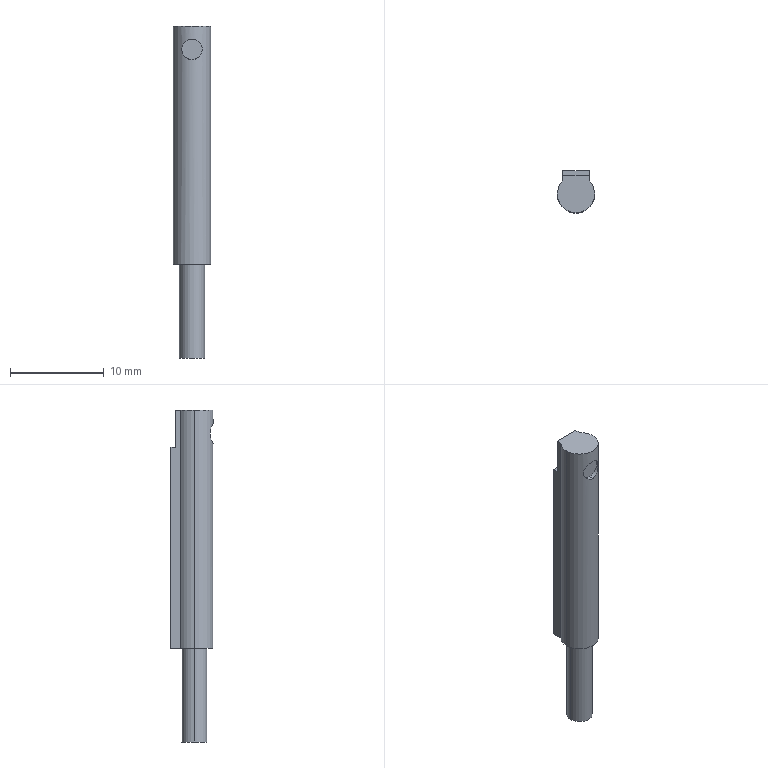Part | STEP file | HI_TD-11-jsn_default | 1 solid | 34 faces | box 4 x 4.5 x 35.5 mm | volume 415.649 mm3 | plane 19 | cylinder 15 | commonest cylinder face diameters 0.6 x4 2.2 x4 4 x3 2.4 x2 2.7 x2